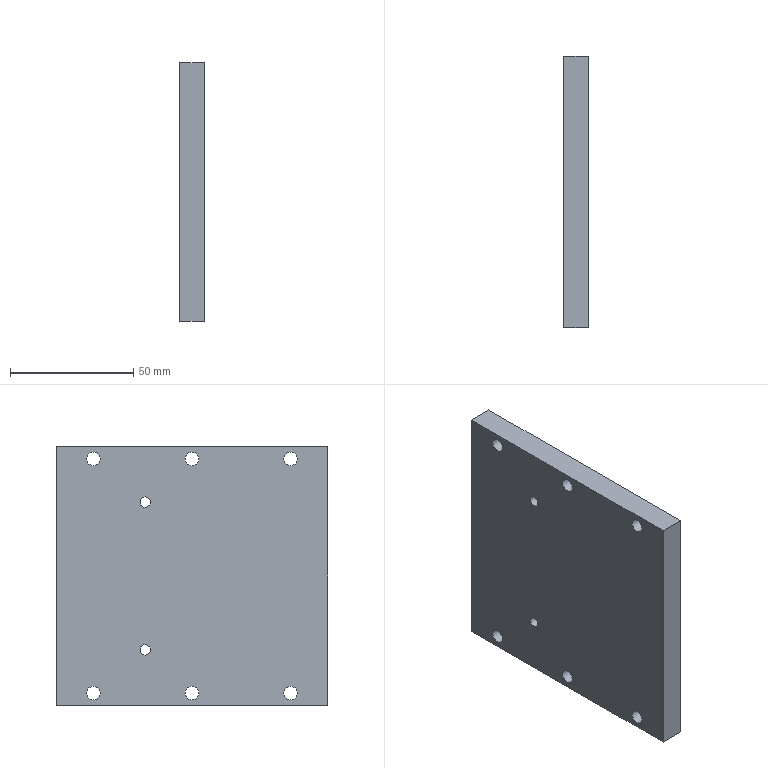Part | NX | 1 solid | 26 faces | box 10 x 110 x 105 mm | volume 112434 mm3 | cylinder 14 | plane 12 | commonest cylinder face diameters 5.5 x6 9 x6 4.2 x2
STEP:
#1=CARTESIAN_POINT('',(0.,-95.,-102.75));
#2=VERTEX_POINT('',#1);
#3=CARTESIAN_POINT('',(0.,-95.,-100.));
#4=DIRECTION('',(1.,0.,0.));
#5=DIRECTION('',(0.,0.,-1.));
#6=AXIS2_PLACEMENT_3D('',#3,#4,#5);
#7=CIRCLE('',#6,2.75);
#8=EDGE_CURVE('',#2,#2,#7,.T.);
#9=ORIENTED_EDGE('',*,*,#8,.F.);
#10=EDGE_LOOP('',(#9));
#11=FACE_BOUND('',#10,.T.);
#12=CARTESIAN_POINT('',(4.3,-95.,-102.75));
#13=VERTEX_POINT('',#12);
#14=CARTESIAN_POINT('',(4.3,-95.,-100.));
#15=DIRECTION('',(-1.,0.,0.));
#16=DIRECTION('',(0.,0.,-1.));
#17=AXIS2_PLACEMENT_3D('',#14,#15,#16);
#18=CIRCLE('',#17,2.75);
#19=EDGE_CURVE('',#13,#13,#18,.T.);
#20=ORIENTED_EDGE('',*,*,#19,.F.);
#21=EDGE_LOOP('',(#20));
#22=FACE_BOUND('',#21,.T.);
#23=CARTESIAN_POINT('',(0.,-95.,-100.));
#24=DIRECTION('',(1.,0.,0.));
#25=DIRECTION('',(0.,0.,1.));
#26=AXIS2_PLACEMENT_3D('',#23,#24,#25);
#27=CYLINDRICAL_SURFACE('',#26,2.75);
#28=ADVANCED_FACE('',(#11,#22),#27,.F.);
#29=CARTESIAN_POINT('',(0.,-55.,-102.75));
#30=VERTEX_POINT('',#29);
#31=CARTESIAN_POINT('',(0.,-55.,-100.));
#32=DIRECTION('',(1.,0.,0.));
#33=DIRECTION('',(0.,0.,-1.));
#34=AXIS2_PLACEMENT_3D('',#31,#32,#33);
#35=CIRCLE('',#34,2.75);
#36=EDGE_CURVE('',#30,#30,#35,.T.);
#37=ORIENTED_EDGE('',*,*,#36,.F.);
#38=EDGE_LOOP('',(#37));
#39=FACE_BOUND('',#38,.T.);
#40=CARTESIAN_POINT('',(4.3,-55.,-102.75));
#41=VERTEX_POINT('',#40);
#42=CARTESIAN_POINT('',(4.3,-55.,-100.));
#43=DIRECTION('',(-1.,0.,0.));
#44=DIRECTION('',(0.,0.,-1.));
#45=AXIS2_PLACEMENT_3D('',#42,#43,#44);
#46=CIRCLE('',#45,2.75);
#47=EDGE_CURVE('',#41,#41,#46,.T.);
#48=ORIENTED_EDGE('',*,*,#47,.F.);
#49=EDGE_LOOP('',(#48));
#50=FACE_BOUND('',#49,.T.);
#51=CARTESIAN_POINT('',(0.,-55.,-100.));
#52=DIRECTION('',(1.,0.,0.));
#53=DIRECTION('',(0.,0.,1.));
#54=AXIS2_PLACEMENT_3D('',#51,#52,#53);
#55=CYLINDRICAL_SURFACE('',#54,2.75);
#56=ADVANCED_FACE('',(#39,#50),#55,.F.);
#57=CARTESIAN_POINT('',(0.,-55.,-7.75));
#58=VERTEX_POINT('',#57);
#59=CARTESIAN_POINT('',(0.,-55.,-5.));
#60=DIRECTION('',(1.,0.,0.));
#61=DIRECTION('',(0.,0.,-1.));
#62=AXIS2_PLACEMENT_3D('',#59,#60,#61);
#63=CIRCLE('',#62,2.75);
#64=EDGE_CURVE('',#58,#58,#63,.T.);
#65=ORIENTED_EDGE('',*,*,#64,.F.);
#66=EDGE_LOOP('',(#65));
#67=FACE_BOUND('',#66,.T.);
#68=CARTESIAN_POINT('',(4.3,-55.,-7.75));
#69=VERTEX_POINT('',#68);
#70=CARTESIAN_POINT('',(4.3,-55.,-5.));
#71=DIRECTION('',(-1.,0.,0.));
#72=DIRECTION('',(0.,0.,-1.));
#73=AXIS2_PLACEMENT_3D('',#70,#71,#72);
#74=CIRCLE('',#73,2.75);
#75=EDGE_CURVE('',#69,#69,#74,.T.);
#76=ORIENTED_EDGE('',*,*,#75,.F.);
#77=EDGE_LOOP('',(#76));
#78=FACE_BOUND('',#77,.T.);
#79=CARTESIAN_POINT('',(0.,-55.,-5.));
#80=DIRECTION('',(1.,0.,0.));
#81=DIRECTION('',(0.,0.,1.));
#82=AXIS2_PLACEMENT_3D('',#79,#80,#81);
#83=CYLINDRICAL_SURFACE('',#82,2.75);
#84=ADVANCED_FACE('',(#67,#78),#83,.F.);
#85=CARTESIAN_POINT('',(0.,-15.,-102.75));
#86=VERTEX_POINT('',#85);
#87=CARTESIAN_POINT('',(0.,-15.,-100.));
#88=DIRECTION('',(1.,0.,0.));
#89=DIRECTION('',(0.,0.,-1.));
#90=AXIS2_PLACEMENT_3D('',#87,#88,#89);
#91=CIRCLE('',#90,2.75);
#92=EDGE_CURVE('',#86,#86,#91,.T.);
#93=ORIENTED_EDGE('',*,*,#92,.F.);
#94=EDGE_LOOP('',(#93));
#95=FACE_BOUND('',#94,.T.);
#96=CARTESIAN_POINT('',(4.3,-15.,-102.75));
#97=VERTEX_POINT('',#96);
#98=CARTESIAN_POINT('',(4.3,-15.,-100.));
#99=DIRECTION('',(-1.,0.,0.));
#100=DIRECTION('',(0.,0.,-1.));
#101=AXIS2_PLACEMENT_3D('',#98,#99,#100);
#102=CIRCLE('',#101,2.75);
#103=EDGE_CURVE('',#97,#97,#102,.T.);
#104=ORIENTED_EDGE('',*,*,#103,.F.);
#105=EDGE_LOOP('',(#104));
#106=FACE_BOUND('',#105,.T.);
#107=CARTESIAN_POINT('',(0.,-15.,-100.));
#108=DIRECTION('',(1.,0.,0.));
#109=DIRECTION('',(0.,0.,1.));
#110=AXIS2_PLACEMENT_3D('',#107,#108,#109);
#111=CYLINDRICAL_SURFACE('',#110,2.75);
#112=ADVANCED_FACE('',(#95,#106),#111,.F.);
#113=CARTESIAN_POINT('',(0.,-95.,-7.75));
#114=VERTEX_POINT('',#113);
#115=CARTESIAN_POINT('',(0.,-95.,-5.));
#116=DIRECTION('',(-1.,0.,0.));
#117=DIRECTION('',(0.,0.,-1.));
#118=AXIS2_PLACEMENT_3D('',#115,#116,#117);
#119=CIRCLE('',#118,2.75);
#120=EDGE_CURVE('',#114,#114,#119,.T.);
#121=ORIENTED_EDGE('',*,*,#120,.T.);
#122=EDGE_LOOP('',(#121));
#123=FACE_BOUND('',#122,.T.);
#124=CARTESIAN_POINT('',(4.3,-95.,-7.75));
#125=VERTEX_POINT('',#124);
#126=CARTESIAN_POINT('',(4.3,-95.,-5.));
#127=DIRECTION('',(1.,0.,0.));
#128=DIRECTION('',(0.,0.,-1.));
#129=AXIS2_PLACEMENT_3D('',#126,#127,#128);
#130=CIRCLE('',#129,2.75);
#131=EDGE_CURVE('',#125,#125,#130,.T.);
#132=ORIENTED_EDGE('',*,*,#131,.T.);
#133=EDGE_LOOP('',(#132));
#134=FACE_BOUND('',#133,.T.);
#135=CARTESIAN_POINT('',(0.,-95.,-5.));
#136=DIRECTION('',(1.,0.,0.));
#137=DIRECTION('',(0.,0.,1.));
#138=AXIS2_PLACEMENT_3D('',#135,#136,#137);
#139=CYLINDRICAL_SURFACE('',#138,2.75);
#140=ADVANCED_FACE('',(#123,#134),#139,.F.);
#141=CARTESIAN_POINT('',(10.,-36.,-84.6));
#142=VERTEX_POINT('',#141);
#143=CARTESIAN_POINT('',(10.,-36.,-82.5));
#144=DIRECTION('',(1.,0.,0.));
#145=DIRECTION('',(0.,0.,-1.));
#146=AXIS2_PLACEMENT_3D('',#143,#144,#145);
#147=CIRCLE('',#146,2.1);
#148=EDGE_CURVE('',#142,#142,#147,.T.);
#149=ORIENTED_EDGE('',*,*,#148,.F.);
#150=EDGE_LOOP('',(#149));
#151=FACE_BOUND('',#150,.T.);
#152=CARTESIAN_POINT('',(10.,-36.,-24.6));
#153=VERTEX_POINT('',#152);
#154=CARTESIAN_POINT('',(10.,-36.,-22.5));
#155=DIRECTION('',(1.,0.,0.));
#156=DIRECTION('',(0.,0.,-1.));
#157=AXIS2_PLACEMENT_3D('',#154,#155,#156);
#158=CIRCLE('',#157,2.1);
#159=EDGE_CURVE('',#153,#153,#158,.T.);
#160=ORIENTED_EDGE('',*,*,#159,.F.);
#161=EDGE_LOOP('',(#160));
#162=FACE_BOUND('',#161,.T.);
#163=CARTESIAN_POINT('',(10.,0.,0.));
#164=VERTEX_POINT('',#163);
#165=CARTESIAN_POINT('',(10.,0.,-105.));
#166=VERTEX_POINT('',#165);
#167=CARTESIAN_POINT('',(10.,0.,0.));
#168=DIRECTION('',(0.,0.,-1.));
#169=VECTOR('',#168,1.);
#170=LINE('',#167,#169);
#171=EDGE_CURVE('',#164,#166,#170,.T.);
#172=ORIENTED_EDGE('',*,*,#171,.F.);
#173=CARTESIAN_POINT('',(10.,-110.,0.));
#174=VERTEX_POINT('',#173);
#175=CARTESIAN_POINT('',(10.,-110.,0.));
#176=DIRECTION('',(0.,1.,0.));
#177=VECTOR('',#176,1.);
#178=LINE('',#175,#177);
#179=EDGE_CURVE('',#174,#164,#178,.T.);
#180=ORIENTED_EDGE('',*,*,#179,.F.);
#181=CARTESIAN_POINT('',(10.,-110.,-105.));
#182=VERTEX_POINT('',#181);
#183=CARTESIAN_POINT('',(10.,-110.,-105.));
#184=DIRECTION('',(0.,0.,1.));
#185=VECTOR('',#184,1.);
#186=LINE('',#183,#185);
#187=EDGE_CURVE('',#182,#174,#186,.T.);
#188=ORIENTED_EDGE('',*,*,#187,.F.);
#189=CARTESIAN_POINT('',(10.,0.,-105.));
#190=DIRECTION('',(0.,-1.,0.));
#191=VECTOR('',#190,1.);
#192=LINE('',#189,#191);
#193=EDGE_CURVE('',#166,#182,#192,.T.);
#194=ORIENTED_EDGE('',*,*,#193,.F.);
#195=EDGE_LOOP('',(#172,#180,#188,#194));
#196=FACE_BOUND('',#195,.T.);
#197=CARTESIAN_POINT('',(10.,-15.,-104.5));
#198=VERTEX_POINT('',#197);
#199=CARTESIAN_POINT('',(10.,-15.,-100.));
#200=DIRECTION('',(1.,0.,0.));
#201=DIRECTION('',(0.,0.,-1.));
#202=AXIS2_PLACEMENT_3D('',#199,#200,#201);
#203=CIRCLE('',#202,4.5);
#204=EDGE_CURVE('',#198,#198,#203,.T.);
#205=ORIENTED_EDGE('',*,*,#204,.F.);
#206=EDGE_LOOP('',(#205));
#207=FACE_BOUND('',#206,.T.);
#208=CARTESIAN_POINT('',(10.,-55.,-9.5));
#209=VERTEX_POINT('',#208);
#210=CARTESIAN_POINT('',(10.,-55.,-5.));
#211=DIRECTION('',(1.,0.,0.));
#212=DIRECTION('',(0.,0.,-1.));
#213=AXIS2_PLACEMENT_3D('',#210,#211,#212);
#214=CIRCLE('',#213,4.5);
#215=EDGE_CURVE('',#209,#209,#214,.T.);
#216=ORIENTED_EDGE('',*,*,#215,.F.);
#217=EDGE_LOOP('',(#216));
#218=FACE_BOUND('',#217,.T.);
#219=CARTESIAN_POINT('',(10.,-55.,-104.5));
#220=VERTEX_POINT('',#219);
#221=CARTESIAN_POINT('',(10.,-55.,-100.));
#222=DIRECTION('',(1.,0.,0.));
#223=DIRECTION('',(0.,0.,-1.));
#224=AXIS2_PLACEMENT_3D('',#221,#222,#223);
#225=CIRCLE('',#224,4.5);
#226=EDGE_CURVE('',#220,#220,#225,.T.);
#227=ORIENTED_EDGE('',*,*,#226,.F.);
#228=EDGE_LOOP('',(#227));
#229=FACE_BOUND('',#228,.T.);
#230=CARTESIAN_POINT('',(10.,-95.,-9.5));
#231=VERTEX_POINT('',#230);
#232=CARTESIAN_POINT('',(10.,-95.,-5.));
#233=DIRECTION('',(1.,0.,0.));
#234=DIRECTION('',(0.,0.,-1.));
#235=AXIS2_PLACEMENT_3D('',#232,#233,#234);
#236=CIRCLE('',#235,4.5);
#237=EDGE_CURVE('',#231,#231,#236,.T.);
#238=ORIENTED_EDGE('',*,*,#237,.F.);
#239=EDGE_LOOP('',(#238));
#240=FACE_BOUND('',#239,.T.);
#241=CARTESIAN_POINT('',(10.,-95.,-104.5));
#242=VERTEX_POINT('',#241);
#243=CARTESIAN_POINT('',(10.,-95.,-100.));
#244=DIRECTION('',(1.,0.,0.));
#245=DIRECTION('',(0.,0.,-1.));
#246=AXIS2_PLACEMENT_3D('',#243,#244,#245);
#247=CIRCLE('',#246,4.5);
#248=EDGE_CURVE('',#242,#242,#247,.T.);
#249=ORIENTED_EDGE('',*,*,#248,.F.);
#250=EDGE_LOOP('',(#249));
#251=FACE_BOUND('',#250,.T.);
#252=CARTESIAN_POINT('',(10.,-15.,-9.5));
#253=VERTEX_POINT('',#252);
#254=CARTESIAN_POINT('',(10.,-15.,-5.));
#255=DIRECTION('',(-1.,0.,0.));
#256=DIRECTION('',(0.,0.,-1.));
#257=AXIS2_PLACEMENT_3D('',#254,#255,#256);
#258=CIRCLE('',#257,4.5);
#259=EDGE_CURVE('',#253,#253,#258,.T.);
#260=ORIENTED_EDGE('',*,*,#259,.T.);
#261=EDGE_LOOP('',(#260));
#262=FACE_BOUND('',#261,.T.);
#263=CARTESIAN_POINT('',(10.,-15.,-5.));
#264=DIRECTION('',(1.,0.,0.));
#265=DIRECTION('',(0.,0.,1.));
#266=AXIS2_PLACEMENT_3D('',#263,#264,#265);
#267=PLANE('',#266);
#268=ADVANCED_FACE('',(#151,#162,#196,#207,#218,#229,#240,#251,#262),#267,.T.);
#269=ORIENTED_EDGE('',*,*,#171,.T.);
#270=CARTESIAN_POINT('',(0.,0.,-105.));
#271=VERTEX_POINT('',#270);
#272=CARTESIAN_POINT('',(0.,0.,-105.));
#273=DIRECTION('',(1.,0.,0.));
#274=VECTOR('',#273,1.);
#275=LINE('',#272,#274);
#276=EDGE_CURVE('',#271,#166,#275,.T.);
#277=ORIENTED_EDGE('',*,*,#276,.F.);
#278=CARTESIAN_POINT('',(0.,0.,0.));
#279=VERTEX_POINT('',#278);
#280=CARTESIAN_POINT('',(0.,0.,0.));
#281=DIRECTION('',(0.,0.,-1.));
#282=VECTOR('',#281,1.);
#283=LINE('',#280,#282);
#284=EDGE_CURVE('',#279,#271,#283,.T.);
#285=ORIENTED_EDGE('',*,*,#284,.F.);
#286=CARTESIAN_POINT('',(0.,0.,0.));
#287=DIRECTION('',(1.,0.,0.));
#288=VECTOR('',#287,1.);
#289=LINE('',#286,#288);
#290=EDGE_CURVE('',#279,#164,#289,.T.);
#291=ORIENTED_EDGE('',*,*,#290,.T.);
#292=EDGE_LOOP('',(#269,#277,#285,#291));
#293=FACE_OUTER_BOUND('',#292,.T.);
#294=CARTESIAN_POINT('',(0.,0.,0.));
#295=DIRECTION('',(0.,-1.,0.));
#296=DIRECTION('',(0.,0.,1.));
#297=AXIS2_PLACEMENT_3D('',#294,#295,#296);
#298=PLANE('',#297);
#299=ADVANCED_FACE('',(#293),#298,.F.);
#300=ORIENTED_EDGE('',*,*,#193,.T.);
#301=CARTESIAN_POINT('',(0.,-110.,-105.));
#302=VERTEX_POINT('',#301);
#303=CARTESIAN_POINT('',(0.,-110.,-105.));
#304=DIRECTION('',(1.,0.,0.));
#305=VECTOR('',#304,1.);
#306=LINE('',#303,#305);
#307=EDGE_CURVE('',#302,#182,#306,.T.);
#308=ORIENTED_EDGE('',*,*,#307,.F.);
#309=CARTESIAN_POINT('',(0.,0.,-105.));
#310=DIRECTION('',(0.,-1.,0.));
#311=VECTOR('',#310,1.);
#312=LINE('',#309,#311);
#313=EDGE_CURVE('',#271,#302,#312,.T.);
#314=ORIENTED_EDGE('',*,*,#313,.F.);
#315=ORIENTED_EDGE('',*,*,#276,.T.);
#316=EDGE_LOOP('',(#300,#308,#314,#315));
#317=FACE_OUTER_BOUND('',#316,.T.);
#318=CARTESIAN_POINT('',(0.,0.,-105.));
#319=DIRECTION('',(0.,0.,1.));
#320=DIRECTION('',(0.,1.,0.));
#321=AXIS2_PLACEMENT_3D('',#318,#319,#320);
#322=PLANE('',#321);
#323=ADVANCED_FACE('',(#317),#322,.F.);
#324=ORIENTED_EDGE('',*,*,#187,.T.);
#325=CARTESIAN_POINT('',(0.,-110.,0.));
#326=VERTEX_POINT('',#325);
#327=CARTESIAN_POINT('',(0.,-110.,0.));
#328=DIRECTION('',(1.,0.,0.));
#329=VECTOR('',#328,1.);
#330=LINE('',#327,#329);
#331=EDGE_CURVE('',#326,#174,#330,.T.);
#332=ORIENTED_EDGE('',*,*,#331,.F.);
#333=CARTESIAN_POINT('',(0.,-110.,-105.));
#334=DIRECTION('',(0.,0.,1.));
#335=VECTOR('',#334,1.);
#336=LINE('',#333,#335);
#337=EDGE_CURVE('',#302,#326,#336,.T.);
#338=ORIENTED_EDGE('',*,*,#337,.F.);
#339=ORIENTED_EDGE('',*,*,#307,.T.);
#340=EDGE_LOOP('',(#324,#332,#338,#339));
#341=FACE_OUTER_BOUND('',#340,.T.);
#342=CARTESIAN_POINT('',(0.,-110.,-105.));
#343=DIRECTION('',(0.,1.,0.));
#344=DIRECTION('',(0.,0.,-1.));
#345=AXIS2_PLACEMENT_3D('',#342,#343,#344);
#346=PLANE('',#345);
#347=ADVANCED_FACE('',(#341),#346,.F.);
#348=ORIENTED_EDGE('',*,*,#148,.T.);
#349=EDGE_LOOP('',(#348));
#350=FACE_BOUND('',#349,.T.);
#351=CARTESIAN_POINT('',(0.,-36.,-84.6));
#352=VERTEX_POINT('',#351);
#353=CARTESIAN_POINT('',(0.,-36.,-82.5));
#354=DIRECTION('',(1.,0.,0.));
#355=DIRECTION('',(0.,0.,-1.));
#356=AXIS2_PLACEMENT_3D('',#353,#354,#355);
#357=CIRCLE('',#356,2.1);
#358=EDGE_CURVE('',#352,#352,#357,.T.);
#359=ORIENTED_EDGE('',*,*,#358,.F.);
#360=EDGE_LOOP('',(#359));
#361=FACE_BOUND('',#360,.T.);
#362=CARTESIAN_POINT('',(0.,-36.,-82.5));
#363=DIRECTION('',(1.,0.,0.));
#364=DIRECTION('',(0.,0.,1.));
#365=AXIS2_PLACEMENT_3D('',#362,#363,#364);
#366=CYLINDRICAL_SURFACE('',#365,2.1);
#367=ADVANCED_FACE('',(#350,#361),#366,.F.);
#368=ORIENTED_EDGE('',*,*,#159,.T.);
#369=EDGE_LOOP('',(#368));
#370=FACE_BOUND('',#369,.T.);
#371=CARTESIAN_POINT('',(0.,-36.,-24.6));
#372=VERTEX_POINT('',#371);
#373=CARTESIAN_POINT('',(0.,-36.,-22.5));
#374=DIRECTION('',(1.,0.,0.));
#375=DIRECTION('',(0.,0.,-1.));
#376=AXIS2_PLACEMENT_3D('',#373,#374,#375);
#377=CIRCLE('',#376,2.1);
#378=EDGE_CURVE('',#372,#372,#377,.T.);
#379=ORIENTED_EDGE('',*,*,#378,.F.);
#380=EDGE_LOOP('',(#379));
#381=FACE_BOUND('',#380,.T.);
#382=CARTESIAN_POINT('',(0.,-36.,-22.5));
#383=DIRECTION('',(1.,0.,0.));
#384=DIRECTION('',(0.,0.,1.));
#385=AXIS2_PLACEMENT_3D('',#382,#383,#384);
#386=CYLINDRICAL_SURFACE('',#385,2.1);
#387=ADVANCED_FACE('',(#370,#381),#386,.F.);
#388=CARTESIAN_POINT('',(4.3,-15.,-2.25));
#389=VERTEX_POINT('',#388);
#390=CARTESIAN_POINT('',(4.3,-15.,-5.));
#391=DIRECTION('',(1.,0.,0.));
#392=DIRECTION('',(0.,0.,1.));
#393=AXIS2_PLACEMENT_3D('',#390,#391,#392);
#394=CIRCLE('',#393,2.75);
#395=EDGE_CURVE('',#389,#389,#394,.T.);
#396=ORIENTED_EDGE('',*,*,#395,.T.);
#397=EDGE_LOOP('',(#396));
#398=FACE_BOUND('',#397,.T.);
#399=CARTESIAN_POINT('',(0.,-15.,-7.75));
#400=VERTEX_POINT('',#399);
#401=CARTESIAN_POINT('',(0.,-15.,-5.));
#402=DIRECTION('',(1.,0.,0.));
#403=DIRECTION('',(0.,0.,-1.));
#404=AXIS2_PLACEMENT_3D('',#401,#402,#403);
#405=CIRCLE('',#404,2.75);
#406=EDGE_CURVE('',#400,#400,#405,.T.);
#407=ORIENTED_EDGE('',*,*,#406,.F.);
#408=EDGE_LOOP('',(#407));
#409=FACE_BOUND('',#408,.T.);
#410=CARTESIAN_POINT('',(0.,-15.,-5.));
#411=DIRECTION('',(1.,0.,0.));
#412=DIRECTION('',(0.,0.,1.));
#413=AXIS2_PLACEMENT_3D('',#410,#411,#412);
#414=CYLINDRICAL_SURFACE('',#413,2.75);
#415=ADVANCED_FACE('',(#398,#409),#414,.F.);
#416=ORIENTED_EDGE('',*,*,#179,.T.);
#417=ORIENTED_EDGE('',*,*,#290,.F.);
#418=CARTESIAN_POINT('',(0.,-110.,0.));
#419=DIRECTION('',(0.,1.,0.));
#420=VECTOR('',#419,1.);
#421=LINE('',#418,#420);
#422=EDGE_CURVE('',#326,#279,#421,.T.);
#423=ORIENTED_EDGE('',*,*,#422,.F.);
#424=ORIENTED_EDGE('',*,*,#331,.T.);
#425=EDGE_LOOP('',(#416,#417,#423,#424));
#426=FACE_OUTER_BOUND('',#425,.T.);
#427=CARTESIAN_POINT('',(0.,-110.,0.));
#428=DIRECTION('',(0.,0.,-1.));
#429=DIRECTION('',(0.,-1.,0.));
#430=AXIS2_PLACEMENT_3D('',#427,#428,#429);
#431=PLANE('',#430);
#432=ADVANCED_FACE('',(#426),#431,.F.);
#433=ORIENTED_EDGE('',*,*,#284,.T.);
#434=ORIENTED_EDGE('',*,*,#313,.T.);
#435=ORIENTED_EDGE('',*,*,#337,.T.);
#436=ORIENTED_EDGE('',*,*,#422,.T.);
#437=EDGE_LOOP('',(#433,#434,#435,#436));
#438=FACE_BOUND('',#437,.T.);
#439=ORIENTED_EDGE('',*,*,#406,.T.);
#440=EDGE_LOOP('',(#439));
#441=FACE_BOUND('',#440,.T.);
#442=ORIENTED_EDGE('',*,*,#92,.T.);
#443=EDGE_LOOP('',(#442));
#444=FACE_BOUND('',#443,.T.);
#445=ORIENTED_EDGE('',*,*,#378,.T.);
#446=EDGE_LOOP('',(#445));
#447=FACE_BOUND('',#446,.T.);
#448=ORIENTED_EDGE('',*,*,#358,.T.);
#449=EDGE_LOOP('',(#448));
#450=FACE_BOUND('',#449,.T.);
#451=ORIENTED_EDGE('',*,*,#64,.T.);
#452=EDGE_LOOP('',(#451));
#453=FACE_BOUND('',#452,.T.);
#454=ORIENTED_EDGE('',*,*,#36,.T.);
#455=EDGE_LOOP('',(#454));
#456=FACE_BOUND('',#455,.T.);
#457=ORIENTED_EDGE('',*,*,#8,.T.);
#458=EDGE_LOOP('',(#457));
#459=FACE_BOUND('',#458,.T.);
#460=ORIENTED_EDGE('',*,*,#120,.F.);
#461=EDGE_LOOP('',(#460));
#462=FACE_BOUND('',#461,.T.);
#463=CARTESIAN_POINT('',(0.,-15.,-5.));
#464=DIRECTION('',(1.,0.,0.));
#465=DIRECTION('',(0.,0.,1.));
#466=AXIS2_PLACEMENT_3D('',#463,#464,#465);
#467=PLANE('',#466);
#468=ADVANCED_FACE('',(#438,#441,#444,#447,#450,#453,#456,#459,#462),#467,.F.);
#469=CARTESIAN_POINT('',(4.3,-15.,-104.5));
#470=VERTEX_POINT('',#469);
#471=CARTESIAN_POINT('',(4.3,-15.,-100.));
#472=DIRECTION('',(-1.,0.,0.));
#473=DIRECTION('',(0.,0.,-1.));
#474=AXIS2_PLACEMENT_3D('',#471,#472,#473);
#475=CIRCLE('',#474,4.5);
#476=EDGE_CURVE('',#470,#470,#475,.T.);
#477=ORIENTED_EDGE('',*,*,#476,.F.);
#478=EDGE_LOOP('',(#477));
#479=FACE_BOUND('',#478,.T.);
#480=ORIENTED_EDGE('',*,*,#103,.T.);
#481=EDGE_LOOP('',(#480));
#482=FACE_BOUND('',#481,.T.);
#483=CARTESIAN_POINT('',(4.3,-15.,-100.));
#484=DIRECTION('',(1.,0.,0.));
#485=DIRECTION('',(0.,0.,1.));
#486=AXIS2_PLACEMENT_3D('',#483,#484,#485);
#487=PLANE('',#486);
#488=ADVANCED_FACE('',(#479,#482),#487,.T.);
#489=ORIENTED_EDGE('',*,*,#204,.T.);
#490=EDGE_LOOP('',(#489));
#491=FACE_BOUND('',#490,.T.);
#492=ORIENTED_EDGE('',*,*,#476,.T.);
#493=EDGE_LOOP('',(#492));
#494=FACE_BOUND('',#493,.T.);
#495=CARTESIAN_POINT('',(4.3,-15.,-100.));
#496=DIRECTION('',(1.,0.,0.));
#497=DIRECTION('',(0.,0.,1.));
#498=AXIS2_PLACEMENT_3D('',#495,#496,#497);
#499=CYLINDRICAL_SURFACE('',#498,4.5);
#500=ADVANCED_FACE('',(#491,#494),#499,.F.);
#501=CARTESIAN_POINT('',(4.3,-55.,-9.5));
#502=VERTEX_POINT('',#501);
#503=CARTESIAN_POINT('',(4.3,-55.,-5.));
#504=DIRECTION('',(-1.,0.,0.));
#505=DIRECTION('',(0.,0.,-1.));
#506=AXIS2_PLACEMENT_3D('',#503,#504,#505);
#507=CIRCLE('',#506,4.5);
#508=EDGE_CURVE('',#502,#502,#507,.T.);
#509=ORIENTED_EDGE('',*,*,#508,.F.);
#510=EDGE_LOOP('',(#509));
#511=FACE_BOUND('',#510,.T.);
#512=ORIENTED_EDGE('',*,*,#75,.T.);
#513=EDGE_LOOP('',(#512));
#514=FACE_BOUND('',#513,.T.);
#515=CARTESIAN_POINT('',(4.3,-55.,-5.));
#516=DIRECTION('',(1.,0.,0.));
#517=DIRECTION('',(0.,0.,1.));
#518=AXIS2_PLACEMENT_3D('',#515,#516,#517);
#519=PLANE('',#518);
#520=ADVANCED_FACE('',(#511,#514),#519,.T.);
#521=ORIENTED_EDGE('',*,*,#215,.T.);
#522=EDGE_LOOP('',(#521));
#523=FACE_BOUND('',#522,.T.);
#524=ORIENTED_EDGE('',*,*,#508,.T.);
#525=EDGE_LOOP('',(#524));
#526=FACE_BOUND('',#525,.T.);
#527=CARTESIAN_POINT('',(4.3,-55.,-5.));
#528=DIRECTION('',(1.,0.,0.));
#529=DIRECTION('',(0.,0.,1.));
#530=AXIS2_PLACEMENT_3D('',#527,#528,#529);
#531=CYLINDRICAL_SURFACE('',#530,4.5);
#532=ADVANCED_FACE('',(#523,#526),#531,.F.);
#533=CARTESIAN_POINT('',(4.3,-55.,-104.5));
#534=VERTEX_POINT('',#533);
#535=CARTESIAN_POINT('',(4.3,-55.,-100.));
#536=DIRECTION('',(-1.,0.,0.));
#537=DIRECTION('',(0.,0.,-1.));
#538=AXIS2_PLACEMENT_3D('',#535,#536,#537);
#539=CIRCLE('',#538,4.5);
#540=EDGE_CURVE('',#534,#534,#539,.T.);
#541=ORIENTED_EDGE('',*,*,#540,.F.);
#542=EDGE_LOOP('',(#541));
#543=FACE_BOUND('',#542,.T.);
#544=ORIENTED_EDGE('',*,*,#47,.T.);
#545=EDGE_LOOP('',(#544));
#546=FACE_BOUND('',#545,.T.);
#547=CARTESIAN_POINT('',(4.3,-55.,-100.));
#548=DIRECTION('',(1.,0.,0.));
#549=DIRECTION('',(0.,0.,1.));
#550=AXIS2_PLACEMENT_3D('',#547,#548,#549);
#551=PLANE('',#550);
#552=ADVANCED_FACE('',(#543,#546),#551,.T.);
#553=ORIENTED_EDGE('',*,*,#226,.T.);
#554=EDGE_LOOP('',(#553));
#555=FACE_BOUND('',#554,.T.);
#556=ORIENTED_EDGE('',*,*,#540,.T.);
#557=EDGE_LOOP('',(#556));
#558=FACE_BOUND('',#557,.T.);
#559=CARTESIAN_POINT('',(4.3,-55.,-100.));
#560=DIRECTION('',(1.,0.,0.));
#561=DIRECTION('',(0.,0.,1.));
#562=AXIS2_PLACEMENT_3D('',#559,#560,#561);
#563=CYLINDRICAL_SURFACE('',#562,4.5);
#564=ADVANCED_FACE('',(#555,#558),#563,.F.);
#565=ORIENTED_EDGE('',*,*,#237,.T.);
#566=EDGE_LOOP('',(#565));
#567=FACE_BOUND('',#566,.T.);
#568=CARTESIAN_POINT('',(4.3,-95.,-9.5));
#569=VERTEX_POINT('',#568);
#570=CARTESIAN_POINT('',(4.3,-95.,-5.));
#571=DIRECTION('',(-1.,0.,0.));
#572=DIRECTION('',(0.,0.,-1.));
#573=AXIS2_PLACEMENT_3D('',#570,#571,#572);
#574=CIRCLE('',#573,4.5);
#575=EDGE_CURVE('',#569,#569,#574,.T.);
#576=ORIENTED_EDGE('',*,*,#575,.T.);
#577=EDGE_LOOP('',(#576));
#578=FACE_BOUND('',#577,.T.);
#579=CARTESIAN_POINT('',(4.3,-95.,-5.));
#580=DIRECTION('',(1.,0.,0.));
#581=DIRECTION('',(0.,0.,1.));
#582=AXIS2_PLACEMENT_3D('',#579,#580,#581);
#583=CYLINDRICAL_SURFACE('',#582,4.5);
#584=ADVANCED_FACE('',(#567,#578),#583,.F.);
#585=ORIENTED_EDGE('',*,*,#131,.F.);
#586=EDGE_LOOP('',(#585));
#587=FACE_BOUND('',#586,.T.);
#588=ORIENTED_EDGE('',*,*,#575,.F.);
#589=EDGE_LOOP('',(#588));
#590=FACE_BOUND('',#589,.T.);
#591=CARTESIAN_POINT('',(4.3,-95.,-5.));
#592=DIRECTION('',(1.,0.,0.));
#593=DIRECTION('',(0.,0.,1.));
#594=AXIS2_PLACEMENT_3D('',#591,#592,#593);
#595=PLANE('',#594);
#596=ADVANCED_FACE('',(#587,#590),#595,.T.);
#597=CARTESIAN_POINT('',(4.3,-95.,-104.5));
#598=VERTEX_POINT('',#597);
#599=CARTESIAN_POINT('',(4.3,-95.,-100.));
#600=DIRECTION('',(-1.,0.,0.));
#601=DIRECTION('',(0.,0.,-1.));
#602=AXIS2_PLACEMENT_3D('',#599,#600,#601);
#603=CIRCLE('',#602,4.5);
#604=EDGE_CURVE('',#598,#598,#603,.T.);
#605=ORIENTED_EDGE('',*,*,#604,.F.);
#606=EDGE_LOOP('',(#605));
#607=FACE_BOUND('',#606,.T.);
#608=ORIENTED_EDGE('',*,*,#19,.T.);
#609=EDGE_LOOP('',(#608));
#610=FACE_BOUND('',#609,.T.);
#611=CARTESIAN_POINT('',(4.3,-95.,-100.));
#612=DIRECTION('',(1.,0.,0.));
#613=DIRECTION('',(0.,0.,1.));
#614=AXIS2_PLACEMENT_3D('',#611,#612,#613);
#615=PLANE('',#614);
#616=ADVANCED_FACE('',(#607,#610),#615,.T.);
#617=ORIENTED_EDGE('',*,*,#248,.T.);
#618=EDGE_LOOP('',(#617));
#619=FACE_BOUND('',#618,.T.);
#620=ORIENTED_EDGE('',*,*,#604,.T.);
#621=EDGE_LOOP('',(#620));
#622=FACE_BOUND('',#621,.T.);
#623=CARTESIAN_POINT('',(4.3,-95.,-100.));
#624=DIRECTION('',(1.,0.,0.));
#625=DIRECTION('',(0.,0.,1.));
#626=AXIS2_PLACEMENT_3D('',#623,#624,#625);
#627=CYLINDRICAL_SURFACE('',#626,4.5);
#628=ADVANCED_FACE('',(#619,#622),#627,.F.);
#629=CARTESIAN_POINT('',(4.3,-15.,-9.5));
#630=VERTEX_POINT('',#629);
#631=CARTESIAN_POINT('',(4.3,-15.,-5.));
#632=DIRECTION('',(1.,0.,0.));
#633=DIRECTION('',(0.,0.,-1.));
#634=AXIS2_PLACEMENT_3D('',#631,#632,#633);
#635=CIRCLE('',#634,4.5);
#636=EDGE_CURVE('',#630,#630,#635,.T.);
#637=ORIENTED_EDGE('',*,*,#636,.T.);
#638=EDGE_LOOP('',(#637));
#639=FACE_BOUND('',#638,.T.);
#640=ORIENTED_EDGE('',*,*,#395,.F.);
#641=EDGE_LOOP('',(#640));
#642=FACE_BOUND('',#641,.T.);
#643=CARTESIAN_POINT('',(4.3,-15.,-5.));
#644=DIRECTION('',(-1.,0.,0.));
#645=DIRECTION('',(0.,0.,-1.));
#646=AXIS2_PLACEMENT_3D('',#643,#644,#645);
#647=PLANE('',#646);
#648=ADVANCED_FACE('',(#639,#642),#647,.F.);
#649=ORIENTED_EDGE('',*,*,#259,.F.);
#650=EDGE_LOOP('',(#649));
#651=FACE_BOUND('',#650,.T.);
#652=ORIENTED_EDGE('',*,*,#636,.F.);
#653=EDGE_LOOP('',(#652));
#654=FACE_BOUND('',#653,.T.);
#655=CARTESIAN_POINT('',(4.3,-15.,-5.));
#656=DIRECTION('',(1.,0.,0.));
#657=DIRECTION('',(0.,0.,1.));
#658=AXIS2_PLACEMENT_3D('',#655,#656,#657);
#659=CYLINDRICAL_SURFACE('',#658,4.5);
#660=ADVANCED_FACE('',(#651,#654),#659,.F.);
#661=CLOSED_SHELL('',(#28,#56,#84,#112,#140,#268,#299,#323,#347,#367,#387,#415,#432,#468,#488,#500,#520,#532,#552,#564,#584,#596,#616,#628,#648,#660));
#662=MANIFOLD_SOLID_BREP('',#661);
#663=(LENGTH_UNIT()NAMED_UNIT(*)SI_UNIT(.MILLI.,.METRE.));
#664=UNCERTAINTY_MEASURE_WITH_UNIT(LENGTH_MEASURE(0.00002),#663,'','');
#665=(NAMED_UNIT(*)PLANE_ANGLE_UNIT()SI_UNIT($,.RADIAN.));
#666=PLANE_ANGLE_MEASURE_WITH_UNIT(PLANE_ANGLE_MEASURE(0.01745),#665);
#667=DIMENSIONAL_EXPONENTS(0.,0.,0.,0.,0.,0.,0.);
#668=(CONVERSION_BASED_UNIT('DEGREE',#666)NAMED_UNIT(#667)PLANE_ANGLE_UNIT());
#669=(NAMED_UNIT(*)SI_UNIT($,.STERADIAN.)SOLID_ANGLE_UNIT());
#670=(GEOMETRIC_REPRESENTATION_CONTEXT(3)GLOBAL_UNCERTAINTY_ASSIGNED_CONTEXT((#664))GLOBAL_UNIT_ASSIGNED_CONTEXT((#663,#668,#669))REPRESENTATION_CONTEXT('',''));
#671=ADVANCED_BREP_SHAPE_REPRESENTATION('',(#662),#670);